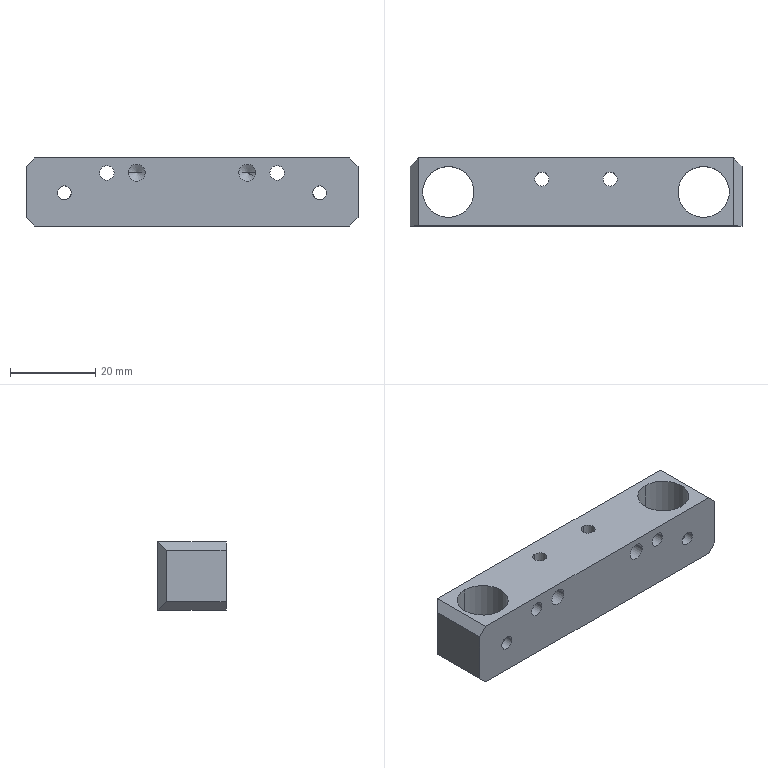Part | 1 solid | 46 faces | box 78 x 16 x 16 mm | volume 15140 mm3 | cylinder 28 | plane 14 | cone 4 | commonest cylinder face diameters 3.3 x12 3.4 x4 4 x4 6 x4 12 x4
STEP:
#1=CARTESIAN_POINT('',(15.,2.,-3.5));
#2=VERTEX_POINT('',#1);
#3=CARTESIAN_POINT('',(11.,2.,-3.5));
#4=VERTEX_POINT('',#3);
#5=CARTESIAN_POINT('',(13.,2.,-3.5));
#6=DIRECTION('',(0.,-1.,0.));
#7=DIRECTION('',(-1.,0.,0.));
#8=AXIS2_PLACEMENT_3D('',#5,#6,#7);
#9=CIRCLE('',#8,2.);
#10=EDGE_CURVE('',#2,#4,#9,.T.);
#11=ORIENTED_EDGE('',*,*,#10,.F.);
#12=CARTESIAN_POINT('',(15.,-8.,-3.5));
#13=VERTEX_POINT('',#12);
#14=CARTESIAN_POINT('',(15.,-8.,-3.5));
#15=DIRECTION('',(0.,-1.,0.));
#16=VECTOR('',#15,1000.);
#17=LINE('',#14,#16);
#18=EDGE_CURVE('',#13,#2,#17,.F.);
#19=ORIENTED_EDGE('',*,*,#18,.F.);
#20=CARTESIAN_POINT('',(11.,-8.,-3.5));
#21=VERTEX_POINT('',#20);
#22=CARTESIAN_POINT('',(13.,-8.,-3.5));
#23=DIRECTION('',(0.,-1.,0.));
#24=DIRECTION('',(-1.,0.,0.));
#25=AXIS2_PLACEMENT_3D('',#22,#23,#24);
#26=CIRCLE('',#25,2.);
#27=EDGE_CURVE('',#13,#21,#26,.T.);
#28=ORIENTED_EDGE('',*,*,#27,.T.);
#29=CARTESIAN_POINT('',(11.,-8.,-3.5));
#30=DIRECTION('',(0.,-1.,0.));
#31=VECTOR('',#30,1000.);
#32=LINE('',#29,#31);
#33=EDGE_CURVE('',#21,#4,#32,.F.);
#34=ORIENTED_EDGE('',*,*,#33,.T.);
#35=EDGE_LOOP('',(#11,#19,#28,#34));
#36=FACE_BOUND('',#35,.T.);
#37=CARTESIAN_POINT('',(13.,-8.,-3.5));
#38=DIRECTION('',(0.,-1.,0.));
#39=DIRECTION('',(1.,0.,0.));
#40=AXIS2_PLACEMENT_3D('',#37,#38,#39);
#41=CYLINDRICAL_SURFACE('',#40,2.);
#42=ADVANCED_FACE('',(#36),#41,.F.);
#43=CARTESIAN_POINT('',(13.,3.202,-3.5));
#44=VERTEX_POINT('',#43);
#45=CARTESIAN_POINT('',(11.,2.,-3.5));
#46=DIRECTION('',(-0.8572,-0.515,0.));
#47=VECTOR('',#46,1000.);
#48=LINE('',#45,#47);
#49=EDGE_CURVE('',#4,#44,#48,.F.);
#50=ORIENTED_EDGE('',*,*,#49,.T.);
#51=CARTESIAN_POINT('',(15.,2.,-3.5));
#52=DIRECTION('',(0.8572,-0.515,0.));
#53=VECTOR('',#52,1000.);
#54=LINE('',#51,#53);
#55=EDGE_CURVE('',#2,#44,#54,.F.);
#56=ORIENTED_EDGE('',*,*,#55,.F.);
#57=ORIENTED_EDGE('',*,*,#10,.T.);
#58=EDGE_LOOP('',(#50,#56,#57));
#59=FACE_BOUND('',#58,.T.);
#60=CARTESIAN_POINT('',(13.,2.,-3.5));
#61=DIRECTION('',(0.,-1.,0.));
#62=DIRECTION('',(1.,0.,0.));
#63=AXIS2_PLACEMENT_3D('',#60,#61,#62);
#64=CONICAL_SURFACE('',#63,2.,1.03);
#65=ADVANCED_FACE('',(#59),#64,.F.);
#66=CARTESIAN_POINT('',(-11.,2.,-3.5));
#67=VERTEX_POINT('',#66);
#68=CARTESIAN_POINT('',(-15.,2.,-3.5));
#69=VERTEX_POINT('',#68);
#70=CARTESIAN_POINT('',(-13.,2.,-3.5));
#71=DIRECTION('',(0.,-1.,0.));
#72=DIRECTION('',(-1.,0.,0.));
#73=AXIS2_PLACEMENT_3D('',#70,#71,#72);
#74=CIRCLE('',#73,2.);
#75=EDGE_CURVE('',#67,#69,#74,.T.);
#76=ORIENTED_EDGE('',*,*,#75,.F.);
#77=CARTESIAN_POINT('',(-11.,-8.,-3.5));
#78=VERTEX_POINT('',#77);
#79=CARTESIAN_POINT('',(-11.,-8.,-3.5));
#80=DIRECTION('',(0.,-1.,0.));
#81=VECTOR('',#80,1000.);
#82=LINE('',#79,#81);
#83=EDGE_CURVE('',#78,#67,#82,.F.);
#84=ORIENTED_EDGE('',*,*,#83,.F.);
#85=CARTESIAN_POINT('',(-15.,-8.,-3.5));
#86=VERTEX_POINT('',#85);
#87=CARTESIAN_POINT('',(-13.,-8.,-3.5));
#88=DIRECTION('',(0.,-1.,0.));
#89=DIRECTION('',(-1.,0.,0.));
#90=AXIS2_PLACEMENT_3D('',#87,#88,#89);
#91=CIRCLE('',#90,2.);
#92=EDGE_CURVE('',#78,#86,#91,.T.);
#93=ORIENTED_EDGE('',*,*,#92,.T.);
#94=CARTESIAN_POINT('',(-15.,-8.,-3.5));
#95=DIRECTION('',(0.,-1.,0.));
#96=VECTOR('',#95,1000.);
#97=LINE('',#94,#96);
#98=EDGE_CURVE('',#86,#69,#97,.F.);
#99=ORIENTED_EDGE('',*,*,#98,.T.);
#100=EDGE_LOOP('',(#76,#84,#93,#99));
#101=FACE_BOUND('',#100,.T.);
#102=CARTESIAN_POINT('',(-13.,-8.,-3.5));
#103=DIRECTION('',(0.,-1.,0.));
#104=DIRECTION('',(1.,0.,0.));
#105=AXIS2_PLACEMENT_3D('',#102,#103,#104);
#106=CYLINDRICAL_SURFACE('',#105,2.);
#107=ADVANCED_FACE('',(#101),#106,.F.);
#108=CARTESIAN_POINT('',(-13.,3.202,-3.5));
#109=VERTEX_POINT('',#108);
#110=CARTESIAN_POINT('',(-15.,2.,-3.5));
#111=DIRECTION('',(-0.8572,-0.515,0.));
#112=VECTOR('',#111,1000.);
#113=LINE('',#110,#112);
#114=EDGE_CURVE('',#69,#109,#113,.F.);
#115=ORIENTED_EDGE('',*,*,#114,.T.);
#116=CARTESIAN_POINT('',(-11.,2.,-3.5));
#117=DIRECTION('',(0.8572,-0.515,0.));
#118=VECTOR('',#117,1000.);
#119=LINE('',#116,#118);
#120=EDGE_CURVE('',#67,#109,#119,.F.);
#121=ORIENTED_EDGE('',*,*,#120,.F.);
#122=ORIENTED_EDGE('',*,*,#75,.T.);
#123=EDGE_LOOP('',(#115,#121,#122));
#124=FACE_BOUND('',#123,.T.);
#125=CARTESIAN_POINT('',(-13.,2.,-3.5));
#126=DIRECTION('',(0.,-1.,0.));
#127=DIRECTION('',(1.,0.,0.));
#128=AXIS2_PLACEMENT_3D('',#125,#126,#127);
#129=CONICAL_SURFACE('',#128,2.,1.03);
#130=ADVANCED_FACE('',(#124),#129,.F.);
#131=CARTESIAN_POINT('',(28.35,5.769,-8.2));
#132=VERTEX_POINT('',#131);
#133=CARTESIAN_POINT('',(30.,6.,-6.55));
#134=VERTEX_POINT('',#133);
#135=CARTESIAN_POINT('',(28.35,5.769,-8.2));
#136=CARTESIAN_POINT('',(28.35,5.769,-7.324));
#137=CARTESIAN_POINT('',(29.124,6.,-6.55));
#138=CARTESIAN_POINT('',(30.,6.,-6.55));
#139=B_SPLINE_CURVE_WITH_KNOTS('',3,(#135,#136,#137,#138),.UNSPECIFIED.,.F.,.F.,(4,4),(0.,0.00259),.UNSPECIFIED.);
#140=EDGE_CURVE('',#132,#134,#139,.T.);
#141=ORIENTED_EDGE('',*,*,#140,.F.);
#142=CARTESIAN_POINT('',(28.35,8.,-8.2));
#143=VERTEX_POINT('',#142);
#144=CARTESIAN_POINT('',(28.35,8.,-8.2));
#145=DIRECTION('',(0.,1.,0.));
#146=VECTOR('',#145,1000.);
#147=LINE('',#144,#146);
#148=EDGE_CURVE('',#143,#132,#147,.F.);
#149=ORIENTED_EDGE('',*,*,#148,.F.);
#150=CARTESIAN_POINT('',(31.65,8.,-8.2));
#151=VERTEX_POINT('',#150);
#152=CARTESIAN_POINT('',(30.,8.,-8.2));
#153=DIRECTION('',(0.,1.,0.));
#154=DIRECTION('',(1.,0.,0.));
#155=AXIS2_PLACEMENT_3D('',#152,#153,#154);
#156=CIRCLE('',#155,1.65);
#157=EDGE_CURVE('',#143,#151,#156,.T.);
#158=ORIENTED_EDGE('',*,*,#157,.T.);
#159=CARTESIAN_POINT('',(31.65,5.769,-8.2));
#160=VERTEX_POINT('',#159);
#161=CARTESIAN_POINT('',(31.65,8.,-8.2));
#162=DIRECTION('',(0.,1.,0.));
#163=VECTOR('',#162,1000.);
#164=LINE('',#161,#163);
#165=EDGE_CURVE('',#151,#160,#164,.F.);
#166=ORIENTED_EDGE('',*,*,#165,.T.);
#167=CARTESIAN_POINT('',(30.,6.,-6.55));
#168=CARTESIAN_POINT('',(30.876,6.,-6.55));
#169=CARTESIAN_POINT('',(31.65,5.769,-7.324));
#170=CARTESIAN_POINT('',(31.65,5.769,-8.2));
#171=B_SPLINE_CURVE_WITH_KNOTS('',3,(#167,#168,#169,#170),.UNSPECIFIED.,.F.,.F.,(4,4),(0.,0.00259),.UNSPECIFIED.);
#172=EDGE_CURVE('',#134,#160,#171,.T.);
#173=ORIENTED_EDGE('',*,*,#172,.F.);
#174=EDGE_LOOP('',(#141,#149,#158,#166,#173));
#175=FACE_BOUND('',#174,.T.);
#176=CARTESIAN_POINT('',(30.,8.,-8.2));
#177=DIRECTION('',(0.,1.,0.));
#178=DIRECTION('',(-1.,0.,0.));
#179=AXIS2_PLACEMENT_3D('',#176,#177,#178);
#180=CYLINDRICAL_SURFACE('',#179,1.65);
#181=ADVANCED_FACE('',(#175),#180,.F.);
#182=CARTESIAN_POINT('',(28.35,-8.,-8.2));
#183=VERTEX_POINT('',#182);
#184=CARTESIAN_POINT('',(31.65,-8.,-8.2));
#185=VERTEX_POINT('',#184);
#186=CARTESIAN_POINT('',(30.,-8.,-8.2));
#187=DIRECTION('',(0.,1.,0.));
#188=DIRECTION('',(1.,0.,0.));
#189=AXIS2_PLACEMENT_3D('',#186,#187,#188);
#190=CIRCLE('',#189,1.65);
#191=EDGE_CURVE('',#183,#185,#190,.T.);
#192=ORIENTED_EDGE('',*,*,#191,.F.);
#193=CARTESIAN_POINT('',(28.35,-5.769,-8.2));
#194=VERTEX_POINT('',#193);
#195=CARTESIAN_POINT('',(28.35,8.,-8.2));
#196=DIRECTION('',(0.,1.,0.));
#197=VECTOR('',#196,1000.);
#198=LINE('',#195,#197);
#199=EDGE_CURVE('',#194,#183,#198,.F.);
#200=ORIENTED_EDGE('',*,*,#199,.F.);
#201=CARTESIAN_POINT('',(30.,-6.,-6.55));
#202=VERTEX_POINT('',#201);
#203=CARTESIAN_POINT('',(30.,-6.,-6.55));
#204=CARTESIAN_POINT('',(29.124,-6.,-6.55));
#205=CARTESIAN_POINT('',(28.35,-5.769,-7.324));
#206=CARTESIAN_POINT('',(28.35,-5.769,-8.2));
#207=B_SPLINE_CURVE_WITH_KNOTS('',3,(#203,#204,#205,#206),.UNSPECIFIED.,.F.,.F.,(4,4),(0.,0.00259),.UNSPECIFIED.);
#208=EDGE_CURVE('',#202,#194,#207,.T.);
#209=ORIENTED_EDGE('',*,*,#208,.F.);
#210=CARTESIAN_POINT('',(31.65,-5.769,-8.2));
#211=VERTEX_POINT('',#210);
#212=CARTESIAN_POINT('',(31.65,-5.769,-8.2));
#213=CARTESIAN_POINT('',(31.65,-5.769,-7.324));
#214=CARTESIAN_POINT('',(30.876,-6.,-6.55));
#215=CARTESIAN_POINT('',(30.,-6.,-6.55));
#216=B_SPLINE_CURVE_WITH_KNOTS('',3,(#212,#213,#214,#215),.UNSPECIFIED.,.F.,.F.,(4,4),(0.,0.00259),.UNSPECIFIED.);
#217=EDGE_CURVE('',#211,#202,#216,.T.);
#218=ORIENTED_EDGE('',*,*,#217,.F.);
#219=CARTESIAN_POINT('',(31.65,8.,-8.2));
#220=DIRECTION('',(0.,1.,0.));
#221=VECTOR('',#220,1000.);
#222=LINE('',#219,#221);
#223=EDGE_CURVE('',#211,#185,#222,.F.);
#224=ORIENTED_EDGE('',*,*,#223,.T.);
#225=EDGE_LOOP('',(#192,#200,#209,#218,#224));
#226=FACE_BOUND('',#225,.T.);
#227=CARTESIAN_POINT('',(30.,8.,-8.2));
#228=DIRECTION('',(0.,1.,0.));
#229=DIRECTION('',(-1.,0.,0.));
#230=AXIS2_PLACEMENT_3D('',#227,#228,#229);
#231=CYLINDRICAL_SURFACE('',#230,1.65);
#232=ADVANCED_FACE('',(#226),#231,.F.);
#233=CARTESIAN_POINT('',(-31.65,5.769,-8.2));
#234=VERTEX_POINT('',#233);
#235=CARTESIAN_POINT('',(-30.,6.,-6.55));
#236=VERTEX_POINT('',#235);
#237=CARTESIAN_POINT('',(-31.65,5.769,-8.2));
#238=CARTESIAN_POINT('',(-31.65,5.769,-7.324));
#239=CARTESIAN_POINT('',(-30.876,6.,-6.55));
#240=CARTESIAN_POINT('',(-30.,6.,-6.55));
#241=B_SPLINE_CURVE_WITH_KNOTS('',3,(#237,#238,#239,#240),.UNSPECIFIED.,.F.,.F.,(4,4),(0.,0.00259),.UNSPECIFIED.);
#242=EDGE_CURVE('',#234,#236,#241,.T.);
#243=ORIENTED_EDGE('',*,*,#242,.F.);
#244=CARTESIAN_POINT('',(-31.65,8.,-8.2));
#245=VERTEX_POINT('',#244);
#246=CARTESIAN_POINT('',(-31.65,8.,-8.2));
#247=DIRECTION('',(0.,1.,0.));
#248=VECTOR('',#247,1000.);
#249=LINE('',#246,#248);
#250=EDGE_CURVE('',#245,#234,#249,.F.);
#251=ORIENTED_EDGE('',*,*,#250,.F.);
#252=CARTESIAN_POINT('',(-28.35,8.,-8.2));
#253=VERTEX_POINT('',#252);
#254=CARTESIAN_POINT('',(-30.,8.,-8.2));
#255=DIRECTION('',(0.,1.,0.));
#256=DIRECTION('',(1.,0.,0.));
#257=AXIS2_PLACEMENT_3D('',#254,#255,#256);
#258=CIRCLE('',#257,1.65);
#259=EDGE_CURVE('',#245,#253,#258,.T.);
#260=ORIENTED_EDGE('',*,*,#259,.T.);
#261=CARTESIAN_POINT('',(-28.35,5.769,-8.2));
#262=VERTEX_POINT('',#261);
#263=CARTESIAN_POINT('',(-28.35,8.,-8.2));
#264=DIRECTION('',(0.,1.,0.));
#265=VECTOR('',#264,1000.);
#266=LINE('',#263,#265);
#267=EDGE_CURVE('',#253,#262,#266,.F.);
#268=ORIENTED_EDGE('',*,*,#267,.T.);
#269=CARTESIAN_POINT('',(-30.,6.,-6.55));
#270=CARTESIAN_POINT('',(-29.124,6.,-6.55));
#271=CARTESIAN_POINT('',(-28.35,5.769,-7.324));
#272=CARTESIAN_POINT('',(-28.35,5.769,-8.2));
#273=B_SPLINE_CURVE_WITH_KNOTS('',3,(#269,#270,#271,#272),.UNSPECIFIED.,.F.,.F.,(4,4),(0.,0.00259),.UNSPECIFIED.);
#274=EDGE_CURVE('',#236,#262,#273,.T.);
#275=ORIENTED_EDGE('',*,*,#274,.F.);
#276=EDGE_LOOP('',(#243,#251,#260,#268,#275));
#277=FACE_BOUND('',#276,.T.);
#278=CARTESIAN_POINT('',(-30.,8.,-8.2));
#279=DIRECTION('',(0.,1.,0.));
#280=DIRECTION('',(-1.,0.,0.));
#281=AXIS2_PLACEMENT_3D('',#278,#279,#280);
#282=CYLINDRICAL_SURFACE('',#281,1.65);
#283=ADVANCED_FACE('',(#277),#282,.F.);
#284=CARTESIAN_POINT('',(-31.65,-8.,-8.2));
#285=VERTEX_POINT('',#284);
#286=CARTESIAN_POINT('',(-28.35,-8.,-8.2));
#287=VERTEX_POINT('',#286);
#288=CARTESIAN_POINT('',(-30.,-8.,-8.2));
#289=DIRECTION('',(0.,1.,0.));
#290=DIRECTION('',(1.,0.,0.));
#291=AXIS2_PLACEMENT_3D('',#288,#289,#290);
#292=CIRCLE('',#291,1.65);
#293=EDGE_CURVE('',#285,#287,#292,.T.);
#294=ORIENTED_EDGE('',*,*,#293,.F.);
#295=CARTESIAN_POINT('',(-31.65,-5.769,-8.2));
#296=VERTEX_POINT('',#295);
#297=CARTESIAN_POINT('',(-31.65,8.,-8.2));
#298=DIRECTION('',(0.,1.,0.));
#299=VECTOR('',#298,1000.);
#300=LINE('',#297,#299);
#301=EDGE_CURVE('',#296,#285,#300,.F.);
#302=ORIENTED_EDGE('',*,*,#301,.F.);
#303=CARTESIAN_POINT('',(-30.,-6.,-6.55));
#304=VERTEX_POINT('',#303);
#305=CARTESIAN_POINT('',(-30.,-6.,-6.55));
#306=CARTESIAN_POINT('',(-30.876,-6.,-6.55));
#307=CARTESIAN_POINT('',(-31.65,-5.769,-7.324));
#308=CARTESIAN_POINT('',(-31.65,-5.769,-8.2));
#309=B_SPLINE_CURVE_WITH_KNOTS('',3,(#305,#306,#307,#308),.UNSPECIFIED.,.F.,.F.,(4,4),(0.,0.00259),.UNSPECIFIED.);
#310=EDGE_CURVE('',#304,#296,#309,.T.);
#311=ORIENTED_EDGE('',*,*,#310,.F.);
#312=CARTESIAN_POINT('',(-28.35,-5.769,-8.2));
#313=VERTEX_POINT('',#312);
#314=CARTESIAN_POINT('',(-28.35,-5.769,-8.2));
#315=CARTESIAN_POINT('',(-28.35,-5.769,-7.324));
#316=CARTESIAN_POINT('',(-29.124,-6.,-6.55));
#317=CARTESIAN_POINT('',(-30.,-6.,-6.55));
#318=B_SPLINE_CURVE_WITH_KNOTS('',3,(#314,#315,#316,#317),.UNSPECIFIED.,.F.,.F.,(4,4),(0.,0.00259),.UNSPECIFIED.);
#319=EDGE_CURVE('',#313,#304,#318,.T.);
#320=ORIENTED_EDGE('',*,*,#319,.F.);
#321=CARTESIAN_POINT('',(-28.35,8.,-8.2));
#322=DIRECTION('',(0.,1.,0.));
#323=VECTOR('',#322,1000.);
#324=LINE('',#321,#323);
#325=EDGE_CURVE('',#313,#287,#324,.F.);
#326=ORIENTED_EDGE('',*,*,#325,.T.);
#327=EDGE_LOOP('',(#294,#302,#311,#320,#326));
#328=FACE_BOUND('',#327,.T.);
#329=CARTESIAN_POINT('',(-30.,8.,-8.2));
#330=DIRECTION('',(0.,1.,0.));
#331=DIRECTION('',(-1.,0.,0.));
#332=AXIS2_PLACEMENT_3D('',#329,#330,#331);
#333=CYLINDRICAL_SURFACE('',#332,1.65);
#334=ADVANCED_FACE('',(#328),#333,.F.);
#335=CARTESIAN_POINT('',(17.,4.6,-3.5));
#336=VERTEX_POINT('',#335);
#337=CARTESIAN_POINT('',(23.,4.6,-3.5));
#338=VERTEX_POINT('',#337);
#339=CARTESIAN_POINT('',(20.,4.6,-3.5));
#340=DIRECTION('',(0.,1.,0.));
#341=DIRECTION('',(1.,0.,0.));
#342=AXIS2_PLACEMENT_3D('',#339,#340,#341);
#343=CIRCLE('',#342,3.);
#344=EDGE_CURVE('',#336,#338,#343,.T.);
#345=ORIENTED_EDGE('',*,*,#344,.F.);
#346=CARTESIAN_POINT('',(17.,8.,-3.5));
#347=VERTEX_POINT('',#346);
#348=CARTESIAN_POINT('',(17.,8.,-3.5));
#349=DIRECTION('',(0.,1.,0.));
#350=VECTOR('',#349,1000.);
#351=LINE('',#348,#350);
#352=EDGE_CURVE('',#347,#336,#351,.F.);
#353=ORIENTED_EDGE('',*,*,#352,.F.);
#354=CARTESIAN_POINT('',(23.,8.,-3.5));
#355=VERTEX_POINT('',#354);
#356=CARTESIAN_POINT('',(20.,8.,-3.5));
#357=DIRECTION('',(0.,1.,0.));
#358=DIRECTION('',(1.,0.,0.));
#359=AXIS2_PLACEMENT_3D('',#356,#357,#358);
#360=CIRCLE('',#359,3.);
#361=EDGE_CURVE('',#347,#355,#360,.T.);
#362=ORIENTED_EDGE('',*,*,#361,.T.);
#363=CARTESIAN_POINT('',(23.,8.,-3.5));
#364=DIRECTION('',(0.,1.,0.));
#365=VECTOR('',#364,1000.);
#366=LINE('',#363,#365);
#367=EDGE_CURVE('',#355,#338,#366,.F.);
#368=ORIENTED_EDGE('',*,*,#367,.T.);
#369=EDGE_LOOP('',(#345,#353,#362,#368));
#370=FACE_BOUND('',#369,.T.);
#371=CARTESIAN_POINT('',(20.,8.,-3.5));
#372=DIRECTION('',(0.,1.,0.));
#373=DIRECTION('',(-1.,0.,0.));
#374=AXIS2_PLACEMENT_3D('',#371,#372,#373);
#375=CYLINDRICAL_SURFACE('',#374,3.);
#376=ADVANCED_FACE('',(#370),#375,.F.);
#377=CARTESIAN_POINT('',(18.3,-8.,-3.5));
#378=VERTEX_POINT('',#377);
#379=CARTESIAN_POINT('',(21.7,-8.,-3.5));
#380=VERTEX_POINT('',#379);
#381=CARTESIAN_POINT('',(20.,-8.,-3.5));
#382=DIRECTION('',(0.,1.,0.));
#383=DIRECTION('',(1.,0.,0.));
#384=AXIS2_PLACEMENT_3D('',#381,#382,#383);
#385=CIRCLE('',#384,1.7);
#386=EDGE_CURVE('',#378,#380,#385,.T.);
#387=ORIENTED_EDGE('',*,*,#386,.F.);
#388=CARTESIAN_POINT('',(18.3,4.6,-3.5));
#389=VERTEX_POINT('',#388);
#390=CARTESIAN_POINT('',(18.3,8.,-3.5));
#391=DIRECTION('',(0.,1.,0.));
#392=VECTOR('',#391,1000.);
#393=LINE('',#390,#392);
#394=EDGE_CURVE('',#389,#378,#393,.F.);
#395=ORIENTED_EDGE('',*,*,#394,.F.);
#396=CARTESIAN_POINT('',(21.7,4.6,-3.5));
#397=VERTEX_POINT('',#396);
#398=CARTESIAN_POINT('',(20.,4.6,-3.5));
#399=DIRECTION('',(0.,1.,0.));
#400=DIRECTION('',(1.,0.,0.));
#401=AXIS2_PLACEMENT_3D('',#398,#399,#400);
#402=CIRCLE('',#401,1.7);
#403=EDGE_CURVE('',#389,#397,#402,.T.);
#404=ORIENTED_EDGE('',*,*,#403,.T.);
#405=CARTESIAN_POINT('',(21.7,8.,-3.5));
#406=DIRECTION('',(0.,1.,0.));
#407=VECTOR('',#406,1000.);
#408=LINE('',#405,#407);
#409=EDGE_CURVE('',#397,#380,#408,.F.);
#410=ORIENTED_EDGE('',*,*,#409,.T.);
#411=EDGE_LOOP('',(#387,#395,#404,#410));
#412=FACE_BOUND('',#411,.T.);
#413=CARTESIAN_POINT('',(20.,8.,-3.5));
#414=DIRECTION('',(0.,1.,0.));
#415=DIRECTION('',(-1.,0.,0.));
#416=AXIS2_PLACEMENT_3D('',#413,#414,#415);
#417=CYLINDRICAL_SURFACE('',#416,1.7);
#418=ADVANCED_FACE('',(#412),#417,.F.);
#419=CARTESIAN_POINT('',(-23.,4.6,-3.5));
#420=VERTEX_POINT('',#419);
#421=CARTESIAN_POINT('',(-17.,4.6,-3.5));
#422=VERTEX_POINT('',#421);
#423=CARTESIAN_POINT('',(-20.,4.6,-3.5));
#424=DIRECTION('',(0.,1.,0.));
#425=DIRECTION('',(1.,0.,0.));
#426=AXIS2_PLACEMENT_3D('',#423,#424,#425);
#427=CIRCLE('',#426,3.);
#428=EDGE_CURVE('',#420,#422,#427,.T.);
#429=ORIENTED_EDGE('',*,*,#428,.F.);
#430=CARTESIAN_POINT('',(-23.,8.,-3.5));
#431=VERTEX_POINT('',#430);
#432=CARTESIAN_POINT('',(-23.,8.,-3.5));
#433=DIRECTION('',(0.,1.,0.));
#434=VECTOR('',#433,1000.);
#435=LINE('',#432,#434);
#436=EDGE_CURVE('',#431,#420,#435,.F.);
#437=ORIENTED_EDGE('',*,*,#436,.F.);
#438=CARTESIAN_POINT('',(-17.,8.,-3.5));
#439=VERTEX_POINT('',#438);
#440=CARTESIAN_POINT('',(-20.,8.,-3.5));
#441=DIRECTION('',(0.,1.,0.));
#442=DIRECTION('',(1.,0.,0.));
#443=AXIS2_PLACEMENT_3D('',#440,#441,#442);
#444=CIRCLE('',#443,3.);
#445=EDGE_CURVE('',#431,#439,#444,.T.);
#446=ORIENTED_EDGE('',*,*,#445,.T.);
#447=CARTESIAN_POINT('',(-17.,8.,-3.5));
#448=DIRECTION('',(0.,1.,0.));
#449=VECTOR('',#448,1000.);
#450=LINE('',#447,#449);
#451=EDGE_CURVE('',#439,#422,#450,.F.);
#452=ORIENTED_EDGE('',*,*,#451,.T.);
#453=EDGE_LOOP('',(#429,#437,#446,#452));
#454=FACE_BOUND('',#453,.T.);
#455=CARTESIAN_POINT('',(-20.,8.,-3.5));
#456=DIRECTION('',(0.,1.,0.));
#457=DIRECTION('',(-1.,0.,0.));
#458=AXIS2_PLACEMENT_3D('',#455,#456,#457);
#459=CYLINDRICAL_SURFACE('',#458,3.);
#460=ADVANCED_FACE('',(#454),#459,.F.);
#461=CARTESIAN_POINT('',(-21.7,-8.,-3.5));
#462=VERTEX_POINT('',#461);
#463=CARTESIAN_POINT('',(-18.3,-8.,-3.5));
#464=VERTEX_POINT('',#463);
#465=CARTESIAN_POINT('',(-20.,-8.,-3.5));
#466=DIRECTION('',(0.,1.,0.));
#467=DIRECTION('',(1.,0.,0.));
#468=AXIS2_PLACEMENT_3D('',#465,#466,#467);
#469=CIRCLE('',#468,1.7);
#470=EDGE_CURVE('',#462,#464,#469,.T.);
#471=ORIENTED_EDGE('',*,*,#470,.F.);
#472=CARTESIAN_POINT('',(-21.7,4.6,-3.5));
#473=VERTEX_POINT('',#472);
#474=CARTESIAN_POINT('',(-21.7,8.,-3.5));
#475=DIRECTION('',(0.,1.,0.));
#476=VECTOR('',#475,1000.);
#477=LINE('',#474,#476);
#478=EDGE_CURVE('',#473,#462,#477,.F.);
#479=ORIENTED_EDGE('',*,*,#478,.F.);
#480=CARTESIAN_POINT('',(-18.3,4.6,-3.5));
#481=VERTEX_POINT('',#480);
#482=CARTESIAN_POINT('',(-20.,4.6,-3.5));
#483=DIRECTION('',(0.,1.,0.));
#484=DIRECTION('',(1.,0.,0.));
#485=AXIS2_PLACEMENT_3D('',#482,#483,#484);
#486=CIRCLE('',#485,1.7);
#487=EDGE_CURVE('',#473,#481,#486,.T.);
#488=ORIENTED_EDGE('',*,*,#487,.T.);
#489=CARTESIAN_POINT('',(-18.3,8.,-3.5));
#490=DIRECTION('',(0.,1.,0.));
#491=VECTOR('',#490,1000.);
#492=LINE('',#489,#491);
#493=EDGE_CURVE('',#481,#464,#492,.F.);
#494=ORIENTED_EDGE('',*,*,#493,.T.);
#495=EDGE_LOOP('',(#471,#479,#488,#494));
#496=FACE_BOUND('',#495,.T.);
#497=CARTESIAN_POINT('',(-20.,8.,-3.5));
#498=DIRECTION('',(0.,1.,0.));
#499=DIRECTION('',(-1.,0.,0.));
#500=AXIS2_PLACEMENT_3D('',#497,#498,#499);
#501=CYLINDRICAL_SURFACE('',#500,1.7);
#502=ADVANCED_FACE('',(#496),#501,.F.);
#503=CARTESIAN_POINT('',(8.,1.35,-16.));
#504=VERTEX_POINT('',#503);
#505=CARTESIAN_POINT('',(8.,4.65,-16.));
#506=VERTEX_POINT('',#505);
#507=CARTESIAN_POINT('',(8.,3.,-16.));
#508=DIRECTION('',(0.,0.,1.));
#509=DIRECTION('',(0.,1.,0.));
#510=AXIS2_PLACEMENT_3D('',#507,#508,#509);
#511=CIRCLE('',#510,1.65);
#512=EDGE_CURVE('',#504,#506,#511,.T.);
#513=ORIENTED_EDGE('',*,*,#512,.F.);
#514=CARTESIAN_POINT('',(8.,1.35,0.));
#515=VERTEX_POINT('',#514);
#516=CARTESIAN_POINT('',(8.,1.35,0.));
#517=DIRECTION('',(0.,0.,1.));
#518=VECTOR('',#517,1000.);
#519=LINE('',#516,#518);
#520=EDGE_CURVE('',#515,#504,#519,.F.);
#521=ORIENTED_EDGE('',*,*,#520,.F.);
#522=CARTESIAN_POINT('',(8.,4.65,0.));
#523=VERTEX_POINT('',#522);
#524=CARTESIAN_POINT('',(8.,3.,0.));
#525=DIRECTION('',(0.,0.,1.));
#526=DIRECTION('',(0.,1.,0.));
#527=AXIS2_PLACEMENT_3D('',#524,#525,#526);
#528=CIRCLE('',#527,1.65);
#529=EDGE_CURVE('',#515,#523,#528,.T.);
#530=ORIENTED_EDGE('',*,*,#529,.T.);
#531=CARTESIAN_POINT('',(8.,4.65,0.));
#532=DIRECTION('',(0.,0.,1.));
#533=VECTOR('',#532,1000.);
#534=LINE('',#531,#533);
#535=EDGE_CURVE('',#523,#506,#534,.F.);
#536=ORIENTED_EDGE('',*,*,#535,.T.);
#537=EDGE_LOOP('',(#513,#521,#530,#536));
#538=FACE_BOUND('',#537,.T.);
#539=CARTESIAN_POINT('',(8.,3.,0.));
#540=DIRECTION('',(0.,0.,1.));
#541=DIRECTION('',(0.,-1.,0.));
#542=AXIS2_PLACEMENT_3D('',#539,#540,#541);
#543=CYLINDRICAL_SURFACE('',#542,1.65);
#544=ADVANCED_FACE('',(#538),#543,.F.);
#545=CARTESIAN_POINT('',(-8.,1.35,-16.));
#546=VERTEX_POINT('',#545);
#547=CARTESIAN_POINT('',(-8.,4.65,-16.));
#548=VERTEX_POINT('',#547);
#549=CARTESIAN_POINT('',(-8.,3.,-16.));
#550=DIRECTION('',(0.,0.,1.));
#551=DIRECTION('',(0.,1.,0.));
#552=AXIS2_PLACEMENT_3D('',#549,#550,#551);
#553=CIRCLE('',#552,1.65);
#554=EDGE_CURVE('',#546,#548,#553,.T.);
#555=ORIENTED_EDGE('',*,*,#554,.F.);
#556=CARTESIAN_POINT('',(-8.,1.35,0.));
#557=VERTEX_POINT('',#556);
#558=CARTESIAN_POINT('',(-8.,1.35,0.));
#559=DIRECTION('',(0.,0.,1.));
#560=VECTOR('',#559,1000.);
#561=LINE('',#558,#560);
#562=EDGE_CURVE('',#557,#546,#561,.F.);
#563=ORIENTED_EDGE('',*,*,#562,.F.);
#564=CARTESIAN_POINT('',(-8.,4.65,0.));
#565=VERTEX_POINT('',#564);
#566=CARTESIAN_POINT('',(-8.,3.,0.));
#567=DIRECTION('',(0.,0.,1.));
#568=DIRECTION('',(0.,1.,0.));
#569=AXIS2_PLACEMENT_3D('',#566,#567,#568);
#570=CIRCLE('',#569,1.65);
#571=EDGE_CURVE('',#557,#565,#570,.T.);
#572=ORIENTED_EDGE('',*,*,#571,.T.);
#573=CARTESIAN_POINT('',(-8.,4.65,0.));
#574=DIRECTION('',(0.,0.,1.));
#575=VECTOR('',#574,1000.);
#576=LINE('',#573,#575);
#577=EDGE_CURVE('',#565,#548,#576,.F.);
#578=ORIENTED_EDGE('',*,*,#577,.T.);
#579=EDGE_LOOP('',(#555,#563,#572,#578));
#580=FACE_BOUND('',#579,.T.);
#581=CARTESIAN_POINT('',(-8.,3.,0.));
#582=DIRECTION('',(0.,0.,1.));
#583=DIRECTION('',(0.,-1.,0.));
#584=AXIS2_PLACEMENT_3D('',#581,#582,#583);
#585=CYLINDRICAL_SURFACE('',#584,1.65);
#586=ADVANCED_FACE('',(#580),#585,.F.);
#587=CARTESIAN_POINT('',(-30.,-6.,-16.));
#588=VERTEX_POINT('',#587);
#589=CARTESIAN_POINT('',(-30.,6.,-16.));
#590=VERTEX_POINT('',#589);
#591=CARTESIAN_POINT('',(-30.,0.,-16.));
#592=DIRECTION('',(0.,0.,1.));
#593=DIRECTION('',(0.,1.,0.));
#594=AXIS2_PLACEMENT_3D('',#591,#592,#593);
#595=CIRCLE('',#594,6.);
#596=EDGE_CURVE('',#588,#590,#595,.T.);
#597=ORIENTED_EDGE('',*,*,#596,.F.);
#598=CARTESIAN_POINT('',(-30.,-6.,-9.85));
#599=VERTEX_POINT('',#598);
#600=CARTESIAN_POINT('',(-30.,-6.,0.));
#601=DIRECTION('',(0.,0.,1.));
#602=VECTOR('',#601,1000.);
#603=LINE('',#600,#602);
#604=EDGE_CURVE('',#599,#588,#603,.F.);
#605=ORIENTED_EDGE('',*,*,#604,.F.);
#606=CARTESIAN_POINT('',(-30.,-6.,-9.85));
#607=CARTESIAN_POINT('',(-29.124,-6.,-9.85));
#608=CARTESIAN_POINT('',(-28.35,-5.769,-9.076));
#609=CARTESIAN_POINT('',(-28.35,-5.769,-8.2));
#610=B_SPLINE_CURVE_WITH_KNOTS('',3,(#606,#607,#608,#609),.UNSPECIFIED.,.F.,.F.,(4,4),(0.,0.00259),.UNSPECIFIED.);
#611=EDGE_CURVE('',#599,#313,#610,.T.);
#612=ORIENTED_EDGE('',*,*,#611,.T.);
#613=ORIENTED_EDGE('',*,*,#319,.T.);
#614=CARTESIAN_POINT('',(-30.,-6.,0.));
#615=VERTEX_POINT('',#614);
#616=CARTESIAN_POINT('',(-30.,-6.,0.));
#617=DIRECTION('',(0.,0.,1.));
#618=VECTOR('',#617,1000.);
#619=LINE('',#616,#618);
#620=EDGE_CURVE('',#304,#615,#619,.T.);
#621=ORIENTED_EDGE('',*,*,#620,.T.);
#622=CARTESIAN_POINT('',(-30.,6.,0.));
#623=VERTEX_POINT('',#622);
#624=CARTESIAN_POINT('',(-30.,0.,0.));
#625=DIRECTION('',(0.,0.,1.));
#626=DIRECTION('',(0.,1.,0.));
#627=AXIS2_PLACEMENT_3D('',#624,#625,#626);
#628=CIRCLE('',#627,6.);
#629=EDGE_CURVE('',#615,#623,#628,.T.);
#630=ORIENTED_EDGE('',*,*,#629,.T.);
#631=CARTESIAN_POINT('',(-30.,6.,0.));
#632=DIRECTION('',(0.,0.,1.));
#633=VECTOR('',#632,1000.);
#634=LINE('',#631,#633);
#635=EDGE_CURVE('',#623,#236,#634,.F.);
#636=ORIENTED_EDGE('',*,*,#635,.T.);
#637=ORIENTED_EDGE('',*,*,#274,.T.);
#638=CARTESIAN_POINT('',(-30.,6.,-9.85));
#639=VERTEX_POINT('',#638);
#640=CARTESIAN_POINT('',(-28.35,5.769,-8.2));
#641=CARTESIAN_POINT('',(-28.35,5.769,-9.076));
#642=CARTESIAN_POINT('',(-29.124,6.,-9.85));
#643=CARTESIAN_POINT('',(-30.,6.,-9.85));
#644=B_SPLINE_CURVE_WITH_KNOTS('',3,(#640,#641,#642,#643),.UNSPECIFIED.,.F.,.F.,(4,4),(0.,0.00259),.UNSPECIFIED.);
#645=EDGE_CURVE('',#262,#639,#644,.T.);
#646=ORIENTED_EDGE('',*,*,#645,.T.);
#647=CARTESIAN_POINT('',(-30.,6.,0.));
#648=DIRECTION('',(0.,0.,1.));
#649=VECTOR('',#648,1000.);
#650=LINE('',#647,#649);
#651=EDGE_CURVE('',#590,#639,#650,.T.);
#652=ORIENTED_EDGE('',*,*,#651,.F.);
#653=EDGE_LOOP('',(#597,#605,#612,#613,#621,#630,#636,#637,#646,#652));
#654=FACE_BOUND('',#653,.T.);
#655=CARTESIAN_POINT('',(-30.,0.,0.));
#656=DIRECTION('',(0.,0.,1.));
#657=DIRECTION('',(0.,-1.,0.));
#658=AXIS2_PLACEMENT_3D('',#655,#656,#657);
#659=CYLINDRICAL_SURFACE('',#658,6.);
#660=ADVANCED_FACE('',(#654),#659,.F.);
#661=CARTESIAN_POINT('',(30.,-6.,-16.));
#662=VERTEX_POINT('',#661);
#663=CARTESIAN_POINT('',(30.,6.,-16.));
#664=VERTEX_POINT('',#663);
#665=CARTESIAN_POINT('',(30.,0.,-16.));
#666=DIRECTION('',(0.,0.,1.));
#667=DIRECTION('',(0.,1.,0.));
#668=AXIS2_PLACEMENT_3D('',#665,#666,#667);
#669=CIRCLE('',#668,6.);
#670=EDGE_CURVE('',#662,#664,#669,.T.);
#671=ORIENTED_EDGE('',*,*,#670,.F.);
#672=CARTESIAN_POINT('',(30.,-6.,-9.85));
#673=VERTEX_POINT('',#672);
#674=CARTESIAN_POINT('',(30.,-6.,0.));
#675=DIRECTION('',(0.,0.,1.));
#676=VECTOR('',#675,1000.);
#677=LINE('',#674,#676);
#678=EDGE_CURVE('',#673,#662,#677,.F.);
#679=ORIENTED_EDGE('',*,*,#678,.F.);
#680=CARTESIAN_POINT('',(30.,-6.,-9.85));
#681=CARTESIAN_POINT('',(30.876,-6.,-9.85));
#682=CARTESIAN_POINT('',(31.65,-5.769,-9.076));
#683=CARTESIAN_POINT('',(31.65,-5.769,-8.2));
#684=B_SPLINE_CURVE_WITH_KNOTS('',3,(#680,#681,#682,#683),.UNSPECIFIED.,.F.,.F.,(4,4),(0.,0.00259),.UNSPECIFIED.);
#685=EDGE_CURVE('',#673,#211,#684,.T.);
#686=ORIENTED_EDGE('',*,*,#685,.T.);
#687=ORIENTED_EDGE('',*,*,#217,.T.);
#688=CARTESIAN_POINT('',(30.,-6.,0.));
#689=VERTEX_POINT('',#688);
#690=CARTESIAN_POINT('',(30.,-6.,0.));
#691=DIRECTION('',(0.,0.,1.));
#692=VECTOR('',#691,1000.);
#693=LINE('',#690,#692);
#694=EDGE_CURVE('',#202,#689,#693,.T.);
#695=ORIENTED_EDGE('',*,*,#694,.T.);
#696=CARTESIAN_POINT('',(30.,6.,0.));
#697=VERTEX_POINT('',#696);
#698=CARTESIAN_POINT('',(30.,0.,0.));
#699=DIRECTION('',(0.,0.,1.));
#700=DIRECTION('',(0.,1.,0.));
#701=AXIS2_PLACEMENT_3D('',#698,#699,#700);
#702=CIRCLE('',#701,6.);
#703=EDGE_CURVE('',#689,#697,#702,.T.);
#704=ORIENTED_EDGE('',*,*,#703,.T.);
#705=CARTESIAN_POINT('',(30.,6.,0.));
#706=DIRECTION('',(0.,0.,1.));
#707=VECTOR('',#706,1000.);
#708=LINE('',#705,#707);
#709=EDGE_CURVE('',#697,#134,#708,.F.);
#710=ORIENTED_EDGE('',*,*,#709,.T.);
#711=ORIENTED_EDGE('',*,*,#172,.T.);
#712=CARTESIAN_POINT('',(30.,6.,-9.85));
#713=VERTEX_POINT('',#712);
#714=CARTESIAN_POINT('',(31.65,5.769,-8.2));
#715=CARTESIAN_POINT('',(31.65,5.769,-9.076));
#716=CARTESIAN_POINT('',(30.876,6.,-9.85));
#717=CARTESIAN_POINT('',(30.,6.,-9.85));
#718=B_SPLINE_CURVE_WITH_KNOTS('',3,(#714,#715,#716,#717),.UNSPECIFIED.,.F.,.F.,(4,4),(0.,0.00259),.UNSPECIFIED.);
#719=EDGE_CURVE('',#160,#713,#718,.T.);
#720=ORIENTED_EDGE('',*,*,#719,.T.);
#721=CARTESIAN_POINT('',(30.,6.,0.));
#722=DIRECTION('',(0.,0.,1.));
#723=VECTOR('',#722,1000.);
#724=LINE('',#721,#723);
#725=EDGE_CURVE('',#664,#713,#724,.T.);
#726=ORIENTED_EDGE('',*,*,#725,.F.);
#727=EDGE_LOOP('',(#671,#679,#686,#687,#695,#704,#710,#711,#720,#726));
#728=FACE_BOUND('',#727,.T.);
#729=CARTESIAN_POINT('',(30.,0.,0.));
#730=DIRECTION('',(0.,0.,1.));
#731=DIRECTION('',(0.,-1.,0.));
#732=AXIS2_PLACEMENT_3D('',#729,#730,#731);
#733=CYLINDRICAL_SURFACE('',#732,6.);
#734=ADVANCED_FACE('',(#728),#733,.F.);
#735=CARTESIAN_POINT('',(-39.,6.,-2.));
#736=VERTEX_POINT('',#735);
#737=CARTESIAN_POINT('',(-39.,6.,-14.));
#738=VERTEX_POINT('',#737);
#739=CARTESIAN_POINT('',(-39.,6.,-16.));
#740=DIRECTION('',(0.,0.,-1.));
#741=VECTOR('',#740,1000.);
#742=LINE('',#739,#741);
#743=EDGE_CURVE('',#736,#738,#742,.T.);
#744=ORIENTED_EDGE('',*,*,#743,.T.);
#745=CARTESIAN_POINT('',(-39.,-8.,-14.));
#746=VERTEX_POINT('',#745);
#747=CARTESIAN_POINT('',(-39.,-8.,-14.));
#748=DIRECTION('',(0.,-1.,0.));
#749=VECTOR('',#748,1000.);
#750=LINE('',#747,#749);
#751=EDGE_CURVE('',#738,#746,#750,.T.);
#752=ORIENTED_EDGE('',*,*,#751,.T.);
#753=CARTESIAN_POINT('',(-39.,-8.,-2.));
#754=VERTEX_POINT('',#753);
#755=CARTESIAN_POINT('',(-39.,-8.,-16.));
#756=DIRECTION('',(0.,0.,1.));
#757=VECTOR('',#756,1000.);
#758=LINE('',#755,#757);
#759=EDGE_CURVE('',#746,#754,#758,.T.);
#760=ORIENTED_EDGE('',*,*,#759,.T.);
#761=CARTESIAN_POINT('',(-39.,8.,-2.));
#762=DIRECTION('',(0.,1.,0.));
#763=VECTOR('',#762,1000.);
#764=LINE('',#761,#763);
#765=EDGE_CURVE('',#754,#736,#764,.T.);
#766=ORIENTED_EDGE('',*,*,#765,.T.);
#767=EDGE_LOOP('',(#744,#752,#760,#766));
#768=FACE_BOUND('',#767,.T.);
#769=CARTESIAN_POINT('',(-39.,8.,-16.));
#770=DIRECTION('',(1.,0.,0.));
#771=DIRECTION('',(0.,1.,0.));
#772=AXIS2_PLACEMENT_3D('',#769,#770,#771);
#773=PLANE('',#772);
#774=ADVANCED_FACE('',(#768),#773,.F.);
#775=CARTESIAN_POINT('',(30.,8.,-8.2));
#776=DIRECTION('',(0.,1.,0.));
#777=DIRECTION('',(1.,0.,0.));
#778=AXIS2_PLACEMENT_3D('',#775,#776,#777);
#779=CIRCLE('',#778,1.65);
#780=EDGE_CURVE('',#151,#143,#779,.T.);
#781=ORIENTED_EDGE('',*,*,#780,.F.);
#782=ORIENTED_EDGE('',*,*,#157,.F.);
#783=EDGE_LOOP('',(#781,#782));
#784=FACE_BOUND('',#783,.T.);
#785=CARTESIAN_POINT('',(-30.,8.,-8.2));
#786=DIRECTION('',(0.,1.,0.));
#787=DIRECTION('',(1.,0.,0.));
#788=AXIS2_PLACEMENT_3D('',#785,#786,#787);
#789=CIRCLE('',#788,1.65);
#790=EDGE_CURVE('',#253,#245,#789,.T.);
#791=ORIENTED_EDGE('',*,*,#790,.F.);
#792=ORIENTED_EDGE('',*,*,#259,.F.);
#793=EDGE_LOOP('',(#791,#792));
#794=FACE_BOUND('',#793,.T.);
#795=CARTESIAN_POINT('',(20.,8.,-3.5));
#796=DIRECTION('',(0.,1.,0.));
#797=DIRECTION('',(1.,0.,0.));
#798=AXIS2_PLACEMENT_3D('',#795,#796,#797);
#799=CIRCLE('',#798,3.);
#800=EDGE_CURVE('',#355,#347,#799,.T.);
#801=ORIENTED_EDGE('',*,*,#800,.F.);
#802=ORIENTED_EDGE('',*,*,#361,.F.);
#803=EDGE_LOOP('',(#801,#802));
#804=FACE_BOUND('',#803,.T.);
#805=CARTESIAN_POINT('',(-20.,8.,-3.5));
#806=DIRECTION('',(0.,1.,0.));
#807=DIRECTION('',(1.,0.,0.));
#808=AXIS2_PLACEMENT_3D('',#805,#806,#807);
#809=CIRCLE('',#808,3.);
#810=EDGE_CURVE('',#439,#431,#809,.T.);
#811=ORIENTED_EDGE('',*,*,#810,.F.);
#812=ORIENTED_EDGE('',*,*,#445,.F.);
#813=EDGE_LOOP('',(#811,#812));
#814=FACE_BOUND('',#813,.T.);
#815=CARTESIAN_POINT('',(-37.,8.,0.));
#816=VERTEX_POINT('',#815);
#817=CARTESIAN_POINT('',(37.,8.,0.));
#818=VERTEX_POINT('',#817);
#819=CARTESIAN_POINT('',(39.,8.,0.));
#820=DIRECTION('',(1.,0.,0.));
#821=VECTOR('',#820,1000.);
#822=LINE('',#819,#821);
#823=EDGE_CURVE('',#816,#818,#822,.T.);
#824=ORIENTED_EDGE('',*,*,#823,.T.);
#825=CARTESIAN_POINT('',(37.,8.,-16.));
#826=VERTEX_POINT('',#825);
#827=CARTESIAN_POINT('',(37.,8.,-16.));
#828=DIRECTION('',(0.,0.,-1.));
#829=VECTOR('',#828,1000.);
#830=LINE('',#827,#829);
#831=EDGE_CURVE('',#818,#826,#830,.T.);
#832=ORIENTED_EDGE('',*,*,#831,.T.);
#833=CARTESIAN_POINT('',(-37.,8.,-16.));
#834=VERTEX_POINT('',#833);
#835=CARTESIAN_POINT('',(39.,8.,-16.));
#836=DIRECTION('',(1.,0.,0.));
#837=VECTOR('',#836,1000.);
#838=LINE('',#835,#837);
#839=EDGE_CURVE('',#834,#826,#838,.T.);
#840=ORIENTED_EDGE('',*,*,#839,.F.);
#841=CARTESIAN_POINT('',(-37.,8.,-16.));
#842=DIRECTION('',(0.,0.,1.));
#843=VECTOR('',#842,1000.);
#844=LINE('',#841,#843);
#845=EDGE_CURVE('',#834,#816,#844,.T.);
#846=ORIENTED_EDGE('',*,*,#845,.T.);
#847=EDGE_LOOP('',(#824,#832,#840,#846));
#848=FACE_BOUND('',#847,.T.);
#849=CARTESIAN_POINT('',(39.,8.,-16.));
#850=DIRECTION('',(0.,-1.,0.));
#851=DIRECTION('',(1.,0.,0.));
#852=AXIS2_PLACEMENT_3D('',#849,#850,#851);
#853=PLANE('',#852);
#854=ADVANCED_FACE('',(#784,#794,#804,#814,#848),#853,.F.);
#855=CARTESIAN_POINT('',(39.,-8.,-14.));
#856=VERTEX_POINT('',#855);
#857=CARTESIAN_POINT('',(39.,-8.,-2.));
#858=VERTEX_POINT('',#857);
#859=CARTESIAN_POINT('',(39.,-8.,-16.));
#860=DIRECTION('',(0.,0.,1.));
#861=VECTOR('',#860,1000.);
#862=LINE('',#859,#861);
#863=EDGE_CURVE('',#856,#858,#862,.T.);
#864=ORIENTED_EDGE('',*,*,#863,.F.);
#865=CARTESIAN_POINT('',(39.,6.,-14.));
#866=VERTEX_POINT('',#865);
#867=CARTESIAN_POINT('',(39.,8.,-14.));
#868=DIRECTION('',(0.,1.,0.));
#869=VECTOR('',#868,1000.);
#870=LINE('',#867,#869);
#871=EDGE_CURVE('',#856,#866,#870,.T.);
#872=ORIENTED_EDGE('',*,*,#871,.T.);
#873=CARTESIAN_POINT('',(39.,6.,-2.));
#874=VERTEX_POINT('',#873);
#875=CARTESIAN_POINT('',(39.,6.,-16.));
#876=DIRECTION('',(0.,0.,1.));
#877=VECTOR('',#876,1000.);
#878=LINE('',#875,#877);
#879=EDGE_CURVE('',#866,#874,#878,.T.);
#880=ORIENTED_EDGE('',*,*,#879,.T.);
#881=CARTESIAN_POINT('',(39.,8.,-2.));
#882=DIRECTION('',(0.,-1.,0.));
#883=VECTOR('',#882,1000.);
#884=LINE('',#881,#883);
#885=EDGE_CURVE('',#874,#858,#884,.T.);
#886=ORIENTED_EDGE('',*,*,#885,.T.);
#887=EDGE_LOOP('',(#864,#872,#880,#886));
#888=FACE_BOUND('',#887,.T.);
#889=CARTESIAN_POINT('',(39.,8.,-16.));
#890=DIRECTION('',(-1.,0.,0.));
#891=DIRECTION('',(0.,-1.,0.));
#892=AXIS2_PLACEMENT_3D('',#889,#890,#891);
#893=PLANE('',#892);
#894=ADVANCED_FACE('',(#888),#893,.F.);
#895=CARTESIAN_POINT('',(13.,-8.,-3.5));
#896=DIRECTION('',(0.,-1.,0.));
#897=DIRECTION('',(-1.,0.,0.));
#898=AXIS2_PLACEMENT_3D('',#895,#896,#897);
#899=CIRCLE('',#898,2.);
#900=EDGE_CURVE('',#21,#13,#899,.T.);
#901=ORIENTED_EDGE('',*,*,#900,.F.);
#902=ORIENTED_EDGE('',*,*,#27,.F.);
#903=EDGE_LOOP('',(#901,#902));
#904=FACE_BOUND('',#903,.T.);
#905=CARTESIAN_POINT('',(-13.,-8.,-3.5));
#906=DIRECTION('',(0.,-1.,0.));
#907=DIRECTION('',(-1.,0.,0.));
#908=AXIS2_PLACEMENT_3D('',#905,#906,#907);
#909=CIRCLE('',#908,2.);
#910=EDGE_CURVE('',#86,#78,#909,.T.);
#911=ORIENTED_EDGE('',*,*,#910,.F.);
#912=ORIENTED_EDGE('',*,*,#92,.F.);
#913=EDGE_LOOP('',(#911,#912));
#914=FACE_BOUND('',#913,.T.);
#915=CARTESIAN_POINT('',(30.,-8.,-8.2));
#916=DIRECTION('',(0.,1.,0.));
#917=DIRECTION('',(1.,0.,0.));
#918=AXIS2_PLACEMENT_3D('',#915,#916,#917);
#919=CIRCLE('',#918,1.65);
#920=EDGE_CURVE('',#185,#183,#919,.T.);
#921=ORIENTED_EDGE('',*,*,#920,.T.);
#922=ORIENTED_EDGE('',*,*,#191,.T.);
#923=EDGE_LOOP('',(#921,#922));
#924=FACE_BOUND('',#923,.T.);
#925=CARTESIAN_POINT('',(-30.,-8.,-8.2));
#926=DIRECTION('',(0.,1.,0.));
#927=DIRECTION('',(1.,0.,0.));
#928=AXIS2_PLACEMENT_3D('',#925,#926,#927);
#929=CIRCLE('',#928,1.65);
#930=EDGE_CURVE('',#287,#285,#929,.T.);
#931=ORIENTED_EDGE('',*,*,#930,.T.);
#932=ORIENTED_EDGE('',*,*,#293,.T.);
#933=EDGE_LOOP('',(#931,#932));
#934=FACE_BOUND('',#933,.T.);
#935=CARTESIAN_POINT('',(20.,-8.,-3.5));
#936=DIRECTION('',(0.,1.,0.));
#937=DIRECTION('',(1.,0.,0.));
#938=AXIS2_PLACEMENT_3D('',#935,#936,#937);
#939=CIRCLE('',#938,1.7);
#940=EDGE_CURVE('',#380,#378,#939,.T.);
#941=ORIENTED_EDGE('',*,*,#940,.T.);
#942=ORIENTED_EDGE('',*,*,#386,.T.);
#943=EDGE_LOOP('',(#941,#942));
#944=FACE_BOUND('',#943,.T.);
#945=CARTESIAN_POINT('',(-20.,-8.,-3.5));
#946=DIRECTION('',(0.,1.,0.));
#947=DIRECTION('',(1.,0.,0.));
#948=AXIS2_PLACEMENT_3D('',#945,#946,#947);
#949=CIRCLE('',#948,1.7);
#950=EDGE_CURVE('',#464,#462,#949,.T.);
#951=ORIENTED_EDGE('',*,*,#950,.T.);
#952=ORIENTED_EDGE('',*,*,#470,.T.);
#953=EDGE_LOOP('',(#951,#952));
#954=FACE_BOUND('',#953,.T.);
#955=CARTESIAN_POINT('',(37.,-8.,-16.));
#956=VERTEX_POINT('',#955);
#957=CARTESIAN_POINT('',(-37.,-8.,-16.));
#958=VERTEX_POINT('',#957);
#959=CARTESIAN_POINT('',(39.,-8.,-16.));
#960=DIRECTION('',(-1.,0.,0.));
#961=VECTOR('',#960,1000.);
#962=LINE('',#959,#961);
#963=EDGE_CURVE('',#956,#958,#962,.T.);
#964=ORIENTED_EDGE('',*,*,#963,.F.);
#965=CARTESIAN_POINT('',(37.,-8.,-16.));
#966=DIRECTION('',(0.7071,0.,0.7071));
#967=VECTOR('',#966,1000.);
#968=LINE('',#965,#967);
#969=EDGE_CURVE('',#956,#856,#968,.T.);
#970=ORIENTED_EDGE('',*,*,#969,.T.);
#971=ORIENTED_EDGE('',*,*,#863,.T.);
#972=CARTESIAN_POINT('',(37.,-8.,0.));
#973=VERTEX_POINT('',#972);
#974=CARTESIAN_POINT('',(39.,-8.,-2.));
#975=DIRECTION('',(-0.7071,0.,0.7071));
#976=VECTOR('',#975,1000.);
#977=LINE('',#974,#976);
#978=EDGE_CURVE('',#858,#973,#977,.T.);
#979=ORIENTED_EDGE('',*,*,#978,.T.);
#980=CARTESIAN_POINT('',(-37.,-8.,0.));
#981=VERTEX_POINT('',#980);
#982=CARTESIAN_POINT('',(39.,-8.,0.));
#983=DIRECTION('',(-1.,0.,0.));
#984=VECTOR('',#983,1000.);
#985=LINE('',#982,#984);
#986=EDGE_CURVE('',#973,#981,#985,.T.);
#987=ORIENTED_EDGE('',*,*,#986,.T.);
#988=CARTESIAN_POINT('',(-39.,-8.,-2.));
#989=DIRECTION('',(-0.7071,0.,-0.7071));
#990=VECTOR('',#989,1000.);
#991=LINE('',#988,#990);
#992=EDGE_CURVE('',#981,#754,#991,.T.);
#993=ORIENTED_EDGE('',*,*,#992,.T.);
#994=ORIENTED_EDGE('',*,*,#759,.F.);
#995=CARTESIAN_POINT('',(-37.,-8.,-16.));
#996=DIRECTION('',(0.7071,0.,-0.7071));
#997=VECTOR('',#996,1000.);
#998=LINE('',#995,#997);
#999=EDGE_CURVE('',#746,#958,#998,.T.);
#1000=ORIENTED_EDGE('',*,*,#999,.T.);
#1001=EDGE_LOOP('',(#964,#970,#971,#979,#987,#993,#994,#1000));
#1002=FACE_BOUND('',#1001,.T.);
#1003=CARTESIAN_POINT('',(39.,-8.,-16.));
#1004=DIRECTION('',(0.,1.,0.));
#1005=DIRECTION('',(-1.,0.,0.));
#1006=AXIS2_PLACEMENT_3D('',#1003,#1004,#1005);
#1007=PLANE('',#1006);
#1008=ADVANCED_FACE('',(#904,#914,#924,#934,#944,#954,#1002),#1007,.F.);
#1009=CARTESIAN_POINT('',(8.,3.,-16.));
#1010=DIRECTION('',(0.,0.,1.));
#1011=DIRECTION('',(0.,1.,0.));
#1012=AXIS2_PLACEMENT_3D('',#1009,#1010,#1011);
#1013=CIRCLE('',#1012,1.65);
#1014=EDGE_CURVE('',#506,#504,#1013,.T.);
#1015=ORIENTED_EDGE('',*,*,#1014,.T.);
#1016=ORIENTED_EDGE('',*,*,#512,.T.);
#1017=EDGE_LOOP('',(#1015,#1016));
#1018=FACE_BOUND('',#1017,.T.);
#1019=CARTESIAN_POINT('',(-8.,3.,-16.));
#1020=DIRECTION('',(0.,0.,1.));
#1021=DIRECTION('',(0.,1.,0.));
#1022=AXIS2_PLACEMENT_3D('',#1019,#1020,#1021);
#1023=CIRCLE('',#1022,1.65);
#1024=EDGE_CURVE('',#548,#546,#1023,.T.);
#1025=ORIENTED_EDGE('',*,*,#1024,.T.);
#1026=ORIENTED_EDGE('',*,*,#554,.T.);
#1027=EDGE_LOOP('',(#1025,#1026));
#1028=FACE_BOUND('',#1027,.T.);
#1029=CARTESIAN_POINT('',(-30.,0.,-16.));
#1030=DIRECTION('',(0.,0.,1.));
#1031=DIRECTION('',(0.,1.,0.));
#1032=AXIS2_PLACEMENT_3D('',#1029,#1030,#1031);
#1033=CIRCLE('',#1032,6.);
#1034=EDGE_CURVE('',#590,#588,#1033,.T.);
#1035=ORIENTED_EDGE('',*,*,#1034,.T.);
#1036=ORIENTED_EDGE('',*,*,#596,.T.);
#1037=EDGE_LOOP('',(#1035,#1036));
#1038=FACE_BOUND('',#1037,.T.);
#1039=CARTESIAN_POINT('',(30.,0.,-16.));
#1040=DIRECTION('',(0.,0.,1.));
#1041=DIRECTION('',(0.,1.,0.));
#1042=AXIS2_PLACEMENT_3D('',#1039,#1040,#1041);
#1043=CIRCLE('',#1042,6.);
#1044=EDGE_CURVE('',#664,#662,#1043,.T.);
#1045=ORIENTED_EDGE('',*,*,#1044,.T.);
#1046=ORIENTED_EDGE('',*,*,#670,.T.);
#1047=EDGE_LOOP('',(#1045,#1046));
#1048=FACE_BOUND('',#1047,.T.);
#1049=ORIENTED_EDGE('',*,*,#839,.T.);
#1050=CARTESIAN_POINT('',(37.,-8.,-16.));
#1051=DIRECTION('',(0.,-1.,0.));
#1052=VECTOR('',#1051,1000.);
#1053=LINE('',#1050,#1052);
#1054=EDGE_CURVE('',#826,#956,#1053,.T.);
#1055=ORIENTED_EDGE('',*,*,#1054,.T.);
#1056=ORIENTED_EDGE('',*,*,#963,.T.);
#1057=CARTESIAN_POINT('',(-37.,8.,-16.));
#1058=DIRECTION('',(0.,1.,0.));
#1059=VECTOR('',#1058,1000.);
#1060=LINE('',#1057,#1059);
#1061=EDGE_CURVE('',#958,#834,#1060,.T.);
#1062=ORIENTED_EDGE('',*,*,#1061,.T.);
#1063=EDGE_LOOP('',(#1049,#1055,#1056,#1062));
#1064=FACE_BOUND('',#1063,.T.);
#1065=CARTESIAN_POINT('',(0.,0.,-16.));
#1066=DIRECTION('',(0.,0.,-1.));
#1067=DIRECTION('',(0.,1.,0.));
#1068=AXIS2_PLACEMENT_3D('',#1065,#1066,#1067);
#1069=PLANE('',#1068);
#1070=ADVANCED_FACE('',(#1018,#1028,#1038,#1048,#1064),#1069,.T.);
#1071=CARTESIAN_POINT('',(8.,3.,0.));
#1072=DIRECTION('',(0.,0.,1.));
#1073=DIRECTION('',(0.,1.,0.));
#1074=AXIS2_PLACEMENT_3D('',#1071,#1072,#1073);
#1075=CIRCLE('',#1074,1.65);
#1076=EDGE_CURVE('',#523,#515,#1075,.T.);
#1077=ORIENTED_EDGE('',*,*,#1076,.F.);
#1078=ORIENTED_EDGE('',*,*,#529,.F.);
#1079=EDGE_LOOP('',(#1077,#1078));
#1080=FACE_BOUND('',#1079,.T.);
#1081=CARTESIAN_POINT('',(-8.,3.,0.));
#1082=DIRECTION('',(0.,0.,1.));
#1083=DIRECTION('',(0.,1.,0.));
#1084=AXIS2_PLACEMENT_3D('',#1081,#1082,#1083);
#1085=CIRCLE('',#1084,1.65);
#1086=EDGE_CURVE('',#565,#557,#1085,.T.);
#1087=ORIENTED_EDGE('',*,*,#1086,.F.);
#1088=ORIENTED_EDGE('',*,*,#571,.F.);
#1089=EDGE_LOOP('',(#1087,#1088));
#1090=FACE_BOUND('',#1089,.T.);
#1091=CARTESIAN_POINT('',(-30.,0.,0.));
#1092=DIRECTION('',(0.,0.,1.));
#1093=DIRECTION('',(0.,1.,0.));
#1094=AXIS2_PLACEMENT_3D('',#1091,#1092,#1093);
#1095=CIRCLE('',#1094,6.);
#1096=EDGE_CURVE('',#623,#615,#1095,.T.);
#1097=ORIENTED_EDGE('',*,*,#1096,.F.);
#1098=ORIENTED_EDGE('',*,*,#629,.F.);
#1099=EDGE_LOOP('',(#1097,#1098));
#1100=FACE_BOUND('',#1099,.T.);
#1101=CARTESIAN_POINT('',(30.,0.,0.));
#1102=DIRECTION('',(0.,0.,1.));
#1103=DIRECTION('',(0.,1.,0.));
#1104=AXIS2_PLACEMENT_3D('',#1101,#1102,#1103);
#1105=CIRCLE('',#1104,6.);
#1106=EDGE_CURVE('',#697,#689,#1105,.T.);
#1107=ORIENTED_EDGE('',*,*,#1106,.F.);
#1108=ORIENTED_EDGE('',*,*,#703,.F.);
#1109=EDGE_LOOP('',(#1107,#1108));
#1110=FACE_BOUND('',#1109,.T.);
#1111=ORIENTED_EDGE('',*,*,#986,.F.);
#1112=CARTESIAN_POINT('',(37.,0.,0.));
#1113=DIRECTION('',(0.,1.,0.));
#1114=VECTOR('',#1113,1000.);
#1115=LINE('',#1112,#1114);
#1116=EDGE_CURVE('',#973,#818,#1115,.T.);
#1117=ORIENTED_EDGE('',*,*,#1116,.T.);
#1118=ORIENTED_EDGE('',*,*,#823,.F.);
#1119=CARTESIAN_POINT('',(-37.,0.,0.));
#1120=DIRECTION('',(0.,-1.,0.));
#1121=VECTOR('',#1120,1000.);
#1122=LINE('',#1119,#1121);
#1123=EDGE_CURVE('',#816,#981,#1122,.T.);
#1124=ORIENTED_EDGE('',*,*,#1123,.T.);
#1125=EDGE_LOOP('',(#1111,#1117,#1118,#1124));
#1126=FACE_BOUND('',#1125,.T.);
#1127=CARTESIAN_POINT('',(0.,0.,0.));
#1128=DIRECTION('',(0.,0.,-1.));
#1129=DIRECTION('',(0.,1.,0.));
#1130=AXIS2_PLACEMENT_3D('',#1127,#1128,#1129);
#1131=PLANE('',#1130);
#1132=ADVANCED_FACE('',(#1080,#1090,#1100,#1110,#1126),#1131,.F.);
#1133=ORIENTED_EDGE('',*,*,#678,.T.);
#1134=ORIENTED_EDGE('',*,*,#1044,.F.);
#1135=ORIENTED_EDGE('',*,*,#725,.T.);
#1136=CARTESIAN_POINT('',(30.,6.,-9.85));
#1137=CARTESIAN_POINT('',(29.124,6.,-9.85));
#1138=CARTESIAN_POINT('',(28.35,5.769,-9.076));
#1139=CARTESIAN_POINT('',(28.35,5.769,-8.2));
#1140=B_SPLINE_CURVE_WITH_KNOTS('',3,(#1136,#1137,#1138,#1139),.UNSPECIFIED.,.F.,.F.,(4,4),(0.,0.00259),.UNSPECIFIED.);
#1141=EDGE_CURVE('',#713,#132,#1140,.T.);
#1142=ORIENTED_EDGE('',*,*,#1141,.T.);
#1143=ORIENTED_EDGE('',*,*,#140,.T.);
#1144=ORIENTED_EDGE('',*,*,#709,.F.);
#1145=ORIENTED_EDGE('',*,*,#1106,.T.);
#1146=ORIENTED_EDGE('',*,*,#694,.F.);
#1147=ORIENTED_EDGE('',*,*,#208,.T.);
#1148=CARTESIAN_POINT('',(28.35,-5.769,-8.2));
#1149=CARTESIAN_POINT('',(28.35,-5.769,-9.076));
#1150=CARTESIAN_POINT('',(29.124,-6.,-9.85));
#1151=CARTESIAN_POINT('',(30.,-6.,-9.85));
#1152=B_SPLINE_CURVE_WITH_KNOTS('',3,(#1148,#1149,#1150,#1151),.UNSPECIFIED.,.F.,.F.,(4,4),(0.,0.00259),.UNSPECIFIED.);
#1153=EDGE_CURVE('',#194,#673,#1152,.T.);
#1154=ORIENTED_EDGE('',*,*,#1153,.T.);
#1155=EDGE_LOOP('',(#1133,#1134,#1135,#1142,#1143,#1144,#1145,#1146,#1147,#1154));
#1156=FACE_BOUND('',#1155,.T.);
#1157=CARTESIAN_POINT('',(30.,0.,0.));
#1158=DIRECTION('',(0.,0.,1.));
#1159=DIRECTION('',(0.,-1.,0.));
#1160=AXIS2_PLACEMENT_3D('',#1157,#1158,#1159);
#1161=CYLINDRICAL_SURFACE('',#1160,6.);
#1162=ADVANCED_FACE('',(#1156),#1161,.F.);
#1163=ORIENTED_EDGE('',*,*,#604,.T.);
#1164=ORIENTED_EDGE('',*,*,#1034,.F.);
#1165=ORIENTED_EDGE('',*,*,#651,.T.);
#1166=CARTESIAN_POINT('',(-30.,6.,-9.85));
#1167=CARTESIAN_POINT('',(-30.876,6.,-9.85));
#1168=CARTESIAN_POINT('',(-31.65,5.769,-9.076));
#1169=CARTESIAN_POINT('',(-31.65,5.769,-8.2));
#1170=B_SPLINE_CURVE_WITH_KNOTS('',3,(#1166,#1167,#1168,#1169),.UNSPECIFIED.,.F.,.F.,(4,4),(0.,0.00259),.UNSPECIFIED.);
#1171=EDGE_CURVE('',#639,#234,#1170,.T.);
#1172=ORIENTED_EDGE('',*,*,#1171,.T.);
#1173=ORIENTED_EDGE('',*,*,#242,.T.);
#1174=ORIENTED_EDGE('',*,*,#635,.F.);
#1175=ORIENTED_EDGE('',*,*,#1096,.T.);
#1176=ORIENTED_EDGE('',*,*,#620,.F.);
#1177=ORIENTED_EDGE('',*,*,#310,.T.);
#1178=CARTESIAN_POINT('',(-31.65,-5.769,-8.2));
#1179=CARTESIAN_POINT('',(-31.65,-5.769,-9.076));
#1180=CARTESIAN_POINT('',(-30.876,-6.,-9.85));
#1181=CARTESIAN_POINT('',(-30.,-6.,-9.85));
#1182=B_SPLINE_CURVE_WITH_KNOTS('',3,(#1178,#1179,#1180,#1181),.UNSPECIFIED.,.F.,.F.,(4,4),(0.,0.00259),.UNSPECIFIED.);
#1183=EDGE_CURVE('',#296,#599,#1182,.T.);
#1184=ORIENTED_EDGE('',*,*,#1183,.T.);
#1185=EDGE_LOOP('',(#1163,#1164,#1165,#1172,#1173,#1174,#1175,#1176,#1177,#1184));
#1186=FACE_BOUND('',#1185,.T.);
#1187=CARTESIAN_POINT('',(-30.,0.,0.));
#1188=DIRECTION('',(0.,0.,1.));
#1189=DIRECTION('',(0.,-1.,0.));
#1190=AXIS2_PLACEMENT_3D('',#1187,#1188,#1189);
#1191=CYLINDRICAL_SURFACE('',#1190,6.);
#1192=ADVANCED_FACE('',(#1186),#1191,.F.);
#1193=ORIENTED_EDGE('',*,*,#562,.T.);
#1194=ORIENTED_EDGE('',*,*,#1024,.F.);
#1195=ORIENTED_EDGE('',*,*,#577,.F.);
#1196=ORIENTED_EDGE('',*,*,#1086,.T.);
#1197=EDGE_LOOP('',(#1193,#1194,#1195,#1196));
#1198=FACE_BOUND('',#1197,.T.);
#1199=CARTESIAN_POINT('',(-8.,3.,0.));
#1200=DIRECTION('',(0.,0.,1.));
#1201=DIRECTION('',(0.,-1.,0.));
#1202=AXIS2_PLACEMENT_3D('',#1199,#1200,#1201);
#1203=CYLINDRICAL_SURFACE('',#1202,1.65);
#1204=ADVANCED_FACE('',(#1198),#1203,.F.);
#1205=ORIENTED_EDGE('',*,*,#520,.T.);
#1206=ORIENTED_EDGE('',*,*,#1014,.F.);
#1207=ORIENTED_EDGE('',*,*,#535,.F.);
#1208=ORIENTED_EDGE('',*,*,#1076,.T.);
#1209=EDGE_LOOP('',(#1205,#1206,#1207,#1208));
#1210=FACE_BOUND('',#1209,.T.);
#1211=CARTESIAN_POINT('',(8.,3.,0.));
#1212=DIRECTION('',(0.,0.,1.));
#1213=DIRECTION('',(0.,-1.,0.));
#1214=AXIS2_PLACEMENT_3D('',#1211,#1212,#1213);
#1215=CYLINDRICAL_SURFACE('',#1214,1.65);
#1216=ADVANCED_FACE('',(#1210),#1215,.F.);
#1217=ORIENTED_EDGE('',*,*,#478,.T.);
#1218=ORIENTED_EDGE('',*,*,#950,.F.);
#1219=ORIENTED_EDGE('',*,*,#493,.F.);
#1220=CARTESIAN_POINT('',(-20.,4.6,-3.5));
#1221=DIRECTION('',(0.,1.,0.));
#1222=DIRECTION('',(1.,0.,0.));
#1223=AXIS2_PLACEMENT_3D('',#1220,#1221,#1222);
#1224=CIRCLE('',#1223,1.7);
#1225=EDGE_CURVE('',#481,#473,#1224,.T.);
#1226=ORIENTED_EDGE('',*,*,#1225,.T.);
#1227=EDGE_LOOP('',(#1217,#1218,#1219,#1226));
#1228=FACE_BOUND('',#1227,.T.);
#1229=CARTESIAN_POINT('',(-20.,8.,-3.5));
#1230=DIRECTION('',(0.,1.,0.));
#1231=DIRECTION('',(-1.,0.,0.));
#1232=AXIS2_PLACEMENT_3D('',#1229,#1230,#1231);
#1233=CYLINDRICAL_SURFACE('',#1232,1.7);
#1234=ADVANCED_FACE('',(#1228),#1233,.F.);
#1235=ORIENTED_EDGE('',*,*,#1225,.F.);
#1236=ORIENTED_EDGE('',*,*,#487,.F.);
#1237=EDGE_LOOP('',(#1235,#1236));
#1238=FACE_BOUND('',#1237,.T.);
#1239=CARTESIAN_POINT('',(-20.,4.6,-3.5));
#1240=DIRECTION('',(0.,1.,0.));
#1241=DIRECTION('',(1.,0.,0.));
#1242=AXIS2_PLACEMENT_3D('',#1239,#1240,#1241);
#1243=CIRCLE('',#1242,3.);
#1244=EDGE_CURVE('',#422,#420,#1243,.T.);
#1245=ORIENTED_EDGE('',*,*,#1244,.T.);
#1246=ORIENTED_EDGE('',*,*,#428,.T.);
#1247=EDGE_LOOP('',(#1245,#1246));
#1248=FACE_BOUND('',#1247,.T.);
#1249=CARTESIAN_POINT('',(-21.7,4.6,-3.5));
#1250=DIRECTION('',(0.,-1.,0.));
#1251=DIRECTION('',(1.,0.,0.));
#1252=AXIS2_PLACEMENT_3D('',#1249,#1250,#1251);
#1253=PLANE('',#1252);
#1254=ADVANCED_FACE('',(#1238,#1248),#1253,.F.);
#1255=ORIENTED_EDGE('',*,*,#436,.T.);
#1256=ORIENTED_EDGE('',*,*,#1244,.F.);
#1257=ORIENTED_EDGE('',*,*,#451,.F.);
#1258=ORIENTED_EDGE('',*,*,#810,.T.);
#1259=EDGE_LOOP('',(#1255,#1256,#1257,#1258));
#1260=FACE_BOUND('',#1259,.T.);
#1261=CARTESIAN_POINT('',(-20.,8.,-3.5));
#1262=DIRECTION('',(0.,1.,0.));
#1263=DIRECTION('',(-1.,0.,0.));
#1264=AXIS2_PLACEMENT_3D('',#1261,#1262,#1263);
#1265=CYLINDRICAL_SURFACE('',#1264,3.);
#1266=ADVANCED_FACE('',(#1260),#1265,.F.);
#1267=ORIENTED_EDGE('',*,*,#394,.T.);
#1268=ORIENTED_EDGE('',*,*,#940,.F.);
#1269=ORIENTED_EDGE('',*,*,#409,.F.);
#1270=CARTESIAN_POINT('',(20.,4.6,-3.5));
#1271=DIRECTION('',(0.,1.,0.));
#1272=DIRECTION('',(1.,0.,0.));
#1273=AXIS2_PLACEMENT_3D('',#1270,#1271,#1272);
#1274=CIRCLE('',#1273,1.7);
#1275=EDGE_CURVE('',#397,#389,#1274,.T.);
#1276=ORIENTED_EDGE('',*,*,#1275,.T.);
#1277=EDGE_LOOP('',(#1267,#1268,#1269,#1276));
#1278=FACE_BOUND('',#1277,.T.);
#1279=CARTESIAN_POINT('',(20.,8.,-3.5));
#1280=DIRECTION('',(0.,1.,0.));
#1281=DIRECTION('',(-1.,0.,0.));
#1282=AXIS2_PLACEMENT_3D('',#1279,#1280,#1281);
#1283=CYLINDRICAL_SURFACE('',#1282,1.7);
#1284=ADVANCED_FACE('',(#1278),#1283,.F.);
#1285=ORIENTED_EDGE('',*,*,#1275,.F.);
#1286=ORIENTED_EDGE('',*,*,#403,.F.);
#1287=EDGE_LOOP('',(#1285,#1286));
#1288=FACE_BOUND('',#1287,.T.);
#1289=CARTESIAN_POINT('',(20.,4.6,-3.5));
#1290=DIRECTION('',(0.,1.,0.));
#1291=DIRECTION('',(1.,0.,0.));
#1292=AXIS2_PLACEMENT_3D('',#1289,#1290,#1291);
#1293=CIRCLE('',#1292,3.);
#1294=EDGE_CURVE('',#338,#336,#1293,.T.);
#1295=ORIENTED_EDGE('',*,*,#1294,.T.);
#1296=ORIENTED_EDGE('',*,*,#344,.T.);
#1297=EDGE_LOOP('',(#1295,#1296));
#1298=FACE_BOUND('',#1297,.T.);
#1299=CARTESIAN_POINT('',(18.3,4.6,-3.5));
#1300=DIRECTION('',(0.,-1.,0.));
#1301=DIRECTION('',(1.,0.,0.));
#1302=AXIS2_PLACEMENT_3D('',#1299,#1300,#1301);
#1303=PLANE('',#1302);
#1304=ADVANCED_FACE('',(#1288,#1298),#1303,.F.);
#1305=ORIENTED_EDGE('',*,*,#352,.T.);
#1306=ORIENTED_EDGE('',*,*,#1294,.F.);
#1307=ORIENTED_EDGE('',*,*,#367,.F.);
#1308=ORIENTED_EDGE('',*,*,#800,.T.);
#1309=EDGE_LOOP('',(#1305,#1306,#1307,#1308));
#1310=FACE_BOUND('',#1309,.T.);
#1311=CARTESIAN_POINT('',(20.,8.,-3.5));
#1312=DIRECTION('',(0.,1.,0.));
#1313=DIRECTION('',(-1.,0.,0.));
#1314=AXIS2_PLACEMENT_3D('',#1311,#1312,#1313);
#1315=CYLINDRICAL_SURFACE('',#1314,3.);
#1316=ADVANCED_FACE('',(#1310),#1315,.F.);
#1317=ORIENTED_EDGE('',*,*,#301,.T.);
#1318=ORIENTED_EDGE('',*,*,#930,.F.);
#1319=ORIENTED_EDGE('',*,*,#325,.F.);
#1320=ORIENTED_EDGE('',*,*,#611,.F.);
#1321=ORIENTED_EDGE('',*,*,#1183,.F.);
#1322=EDGE_LOOP('',(#1317,#1318,#1319,#1320,#1321));
#1323=FACE_BOUND('',#1322,.T.);
#1324=CARTESIAN_POINT('',(-30.,8.,-8.2));
#1325=DIRECTION('',(0.,1.,0.));
#1326=DIRECTION('',(-1.,0.,0.));
#1327=AXIS2_PLACEMENT_3D('',#1324,#1325,#1326);
#1328=CYLINDRICAL_SURFACE('',#1327,1.65);
#1329=ADVANCED_FACE('',(#1323),#1328,.F.);
#1330=ORIENTED_EDGE('',*,*,#250,.T.);
#1331=ORIENTED_EDGE('',*,*,#1171,.F.);
#1332=ORIENTED_EDGE('',*,*,#645,.F.);
#1333=ORIENTED_EDGE('',*,*,#267,.F.);
#1334=ORIENTED_EDGE('',*,*,#790,.T.);
#1335=EDGE_LOOP('',(#1330,#1331,#1332,#1333,#1334));
#1336=FACE_BOUND('',#1335,.T.);
#1337=CARTESIAN_POINT('',(-30.,8.,-8.2));
#1338=DIRECTION('',(0.,1.,0.));
#1339=DIRECTION('',(-1.,0.,0.));
#1340=AXIS2_PLACEMENT_3D('',#1337,#1338,#1339);
#1341=CYLINDRICAL_SURFACE('',#1340,1.65);
#1342=ADVANCED_FACE('',(#1336),#1341,.F.);
#1343=ORIENTED_EDGE('',*,*,#199,.T.);
#1344=ORIENTED_EDGE('',*,*,#920,.F.);
#1345=ORIENTED_EDGE('',*,*,#223,.F.);
#1346=ORIENTED_EDGE('',*,*,#685,.F.);
#1347=ORIENTED_EDGE('',*,*,#1153,.F.);
#1348=EDGE_LOOP('',(#1343,#1344,#1345,#1346,#1347));
#1349=FACE_BOUND('',#1348,.T.);
#1350=CARTESIAN_POINT('',(30.,8.,-8.2));
#1351=DIRECTION('',(0.,1.,0.));
#1352=DIRECTION('',(-1.,0.,0.));
#1353=AXIS2_PLACEMENT_3D('',#1350,#1351,#1352);
#1354=CYLINDRICAL_SURFACE('',#1353,1.65);
#1355=ADVANCED_FACE('',(#1349),#1354,.F.);
#1356=ORIENTED_EDGE('',*,*,#148,.T.);
#1357=ORIENTED_EDGE('',*,*,#1141,.F.);
#1358=ORIENTED_EDGE('',*,*,#719,.F.);
#1359=ORIENTED_EDGE('',*,*,#165,.F.);
#1360=ORIENTED_EDGE('',*,*,#780,.T.);
#1361=EDGE_LOOP('',(#1356,#1357,#1358,#1359,#1360));
#1362=FACE_BOUND('',#1361,.T.);
#1363=CARTESIAN_POINT('',(30.,8.,-8.2));
#1364=DIRECTION('',(0.,1.,0.));
#1365=DIRECTION('',(-1.,0.,0.));
#1366=AXIS2_PLACEMENT_3D('',#1363,#1364,#1365);
#1367=CYLINDRICAL_SURFACE('',#1366,1.65);
#1368=ADVANCED_FACE('',(#1362),#1367,.F.);
#1369=ORIENTED_EDGE('',*,*,#120,.T.);
#1370=ORIENTED_EDGE('',*,*,#114,.F.);
#1371=CARTESIAN_POINT('',(-13.,2.,-3.5));
#1372=DIRECTION('',(0.,-1.,0.));
#1373=DIRECTION('',(-1.,0.,0.));
#1374=AXIS2_PLACEMENT_3D('',#1371,#1372,#1373);
#1375=CIRCLE('',#1374,2.);
#1376=EDGE_CURVE('',#69,#67,#1375,.T.);
#1377=ORIENTED_EDGE('',*,*,#1376,.T.);
#1378=EDGE_LOOP('',(#1369,#1370,#1377));
#1379=FACE_BOUND('',#1378,.T.);
#1380=CARTESIAN_POINT('',(-13.,2.,-3.5));
#1381=DIRECTION('',(0.,-1.,0.));
#1382=DIRECTION('',(1.,0.,0.));
#1383=AXIS2_PLACEMENT_3D('',#1380,#1381,#1382);
#1384=CONICAL_SURFACE('',#1383,2.,1.03);
#1385=ADVANCED_FACE('',(#1379),#1384,.F.);
#1386=ORIENTED_EDGE('',*,*,#83,.T.);
#1387=ORIENTED_EDGE('',*,*,#1376,.F.);
#1388=ORIENTED_EDGE('',*,*,#98,.F.);
#1389=ORIENTED_EDGE('',*,*,#910,.T.);
#1390=EDGE_LOOP('',(#1386,#1387,#1388,#1389));
#1391=FACE_BOUND('',#1390,.T.);
#1392=CARTESIAN_POINT('',(-13.,-8.,-3.5));
#1393=DIRECTION('',(0.,-1.,0.));
#1394=DIRECTION('',(1.,0.,0.));
#1395=AXIS2_PLACEMENT_3D('',#1392,#1393,#1394);
#1396=CYLINDRICAL_SURFACE('',#1395,2.);
#1397=ADVANCED_FACE('',(#1391),#1396,.F.);
#1398=ORIENTED_EDGE('',*,*,#55,.T.);
#1399=ORIENTED_EDGE('',*,*,#49,.F.);
#1400=CARTESIAN_POINT('',(13.,2.,-3.5));
#1401=DIRECTION('',(0.,-1.,0.));
#1402=DIRECTION('',(-1.,0.,0.));
#1403=AXIS2_PLACEMENT_3D('',#1400,#1401,#1402);
#1404=CIRCLE('',#1403,2.);
#1405=EDGE_CURVE('',#4,#2,#1404,.T.);
#1406=ORIENTED_EDGE('',*,*,#1405,.T.);
#1407=EDGE_LOOP('',(#1398,#1399,#1406));
#1408=FACE_BOUND('',#1407,.T.);
#1409=CARTESIAN_POINT('',(13.,2.,-3.5));
#1410=DIRECTION('',(0.,-1.,0.));
#1411=DIRECTION('',(1.,0.,0.));
#1412=AXIS2_PLACEMENT_3D('',#1409,#1410,#1411);
#1413=CONICAL_SURFACE('',#1412,2.,1.03);
#1414=ADVANCED_FACE('',(#1408),#1413,.F.);
#1415=ORIENTED_EDGE('',*,*,#18,.T.);
#1416=ORIENTED_EDGE('',*,*,#1405,.F.);
#1417=ORIENTED_EDGE('',*,*,#33,.F.);
#1418=ORIENTED_EDGE('',*,*,#900,.T.);
#1419=EDGE_LOOP('',(#1415,#1416,#1417,#1418));
#1420=FACE_BOUND('',#1419,.T.);
#1421=CARTESIAN_POINT('',(13.,-8.,-3.5));
#1422=DIRECTION('',(0.,-1.,0.));
#1423=DIRECTION('',(1.,0.,0.));
#1424=AXIS2_PLACEMENT_3D('',#1421,#1422,#1423);
#1425=CYLINDRICAL_SURFACE('',#1424,2.);
#1426=ADVANCED_FACE('',(#1420),#1425,.F.);
#1427=ORIENTED_EDGE('',*,*,#978,.F.);
#1428=ORIENTED_EDGE('',*,*,#885,.F.);
#1429=CARTESIAN_POINT('',(43.667,1.333,-6.667));
#1430=DIRECTION('',(0.5774,-0.5774,-0.5774));
#1431=VECTOR('',#1430,1000.);
#1432=LINE('',#1429,#1431);
#1433=EDGE_CURVE('',#818,#874,#1432,.T.);
#1434=ORIENTED_EDGE('',*,*,#1433,.F.);
#1435=ORIENTED_EDGE('',*,*,#1116,.F.);
#1436=EDGE_LOOP('',(#1427,#1428,#1434,#1435));
#1437=FACE_BOUND('',#1436,.T.);
#1438=CARTESIAN_POINT('',(39.,8.,-2.));
#1439=DIRECTION('',(-0.7071,0.,-0.7071));
#1440=DIRECTION('',(0.,1.,0.));
#1441=AXIS2_PLACEMENT_3D('',#1438,#1439,#1440);
#1442=PLANE('',#1441);
#1443=ADVANCED_FACE('',(#1437),#1442,.F.);
#1444=ORIENTED_EDGE('',*,*,#1433,.T.);
#1445=ORIENTED_EDGE('',*,*,#879,.F.);
#1446=CARTESIAN_POINT('',(38.333,6.667,-14.667));
#1447=DIRECTION('',(0.5774,-0.5774,0.5774));
#1448=VECTOR('',#1447,1000.);
#1449=LINE('',#1446,#1448);
#1450=EDGE_CURVE('',#826,#866,#1449,.T.);
#1451=ORIENTED_EDGE('',*,*,#1450,.F.);
#1452=ORIENTED_EDGE('',*,*,#831,.F.);
#1453=EDGE_LOOP('',(#1444,#1445,#1451,#1452));
#1454=FACE_BOUND('',#1453,.T.);
#1455=CARTESIAN_POINT('',(39.,6.,-16.));
#1456=DIRECTION('',(-0.7071,-0.7071,0.));
#1457=DIRECTION('',(0.,0.,-1.));
#1458=AXIS2_PLACEMENT_3D('',#1455,#1456,#1457);
#1459=PLANE('',#1458);
#1460=ADVANCED_FACE('',(#1454),#1459,.F.);
#1461=ORIENTED_EDGE('',*,*,#1450,.T.);
#1462=ORIENTED_EDGE('',*,*,#871,.F.);
#1463=ORIENTED_EDGE('',*,*,#969,.F.);
#1464=ORIENTED_EDGE('',*,*,#1054,.F.);
#1465=EDGE_LOOP('',(#1461,#1462,#1463,#1464));
#1466=FACE_BOUND('',#1465,.T.);
#1467=CARTESIAN_POINT('',(37.,0.,-16.));
#1468=DIRECTION('',(0.7071,0.,-0.7071));
#1469=DIRECTION('',(0.,-1.,0.));
#1470=AXIS2_PLACEMENT_3D('',#1467,#1468,#1469);
#1471=PLANE('',#1470);
#1472=ADVANCED_FACE('',(#1466),#1471,.T.);
#1473=ORIENTED_EDGE('',*,*,#992,.F.);
#1474=ORIENTED_EDGE('',*,*,#1123,.F.);
#1475=CARTESIAN_POINT('',(-42.333,2.667,-5.333));
#1476=DIRECTION('',(0.5774,0.5774,0.5774));
#1477=VECTOR('',#1476,1000.);
#1478=LINE('',#1475,#1477);
#1479=EDGE_CURVE('',#736,#816,#1478,.T.);
#1480=ORIENTED_EDGE('',*,*,#1479,.F.);
#1481=ORIENTED_EDGE('',*,*,#765,.F.);
#1482=EDGE_LOOP('',(#1473,#1474,#1480,#1481));
#1483=FACE_BOUND('',#1482,.T.);
#1484=CARTESIAN_POINT('',(-39.,8.,-2.));
#1485=DIRECTION('',(0.7071,0.,-0.7071));
#1486=DIRECTION('',(0.,-1.,0.));
#1487=AXIS2_PLACEMENT_3D('',#1484,#1485,#1486);
#1488=PLANE('',#1487);
#1489=ADVANCED_FACE('',(#1483),#1488,.F.);
#1490=ORIENTED_EDGE('',*,*,#1479,.T.);
#1491=ORIENTED_EDGE('',*,*,#845,.F.);
#1492=CARTESIAN_POINT('',(-37.,8.,-16.));
#1493=DIRECTION('',(0.5774,0.5774,-0.5774));
#1494=VECTOR('',#1493,1000.);
#1495=LINE('',#1492,#1494);
#1496=EDGE_CURVE('',#738,#834,#1495,.T.);
#1497=ORIENTED_EDGE('',*,*,#1496,.F.);
#1498=ORIENTED_EDGE('',*,*,#743,.F.);
#1499=EDGE_LOOP('',(#1490,#1491,#1497,#1498));
#1500=FACE_BOUND('',#1499,.T.);
#1501=CARTESIAN_POINT('',(-37.,8.,-16.));
#1502=DIRECTION('',(0.7071,-0.7071,0.));
#1503=DIRECTION('',(0.,0.,-1.));
#1504=AXIS2_PLACEMENT_3D('',#1501,#1502,#1503);
#1505=PLANE('',#1504);
#1506=ADVANCED_FACE('',(#1500),#1505,.F.);
#1507=ORIENTED_EDGE('',*,*,#999,.F.);
#1508=ORIENTED_EDGE('',*,*,#751,.F.);
#1509=ORIENTED_EDGE('',*,*,#1496,.T.);
#1510=ORIENTED_EDGE('',*,*,#1061,.F.);
#1511=EDGE_LOOP('',(#1507,#1508,#1509,#1510));
#1512=FACE_BOUND('',#1511,.T.);
#1513=CARTESIAN_POINT('',(-37.,0.,-16.));
#1514=DIRECTION('',(-0.7071,0.,-0.7071));
#1515=DIRECTION('',(0.,1.,0.));
#1516=AXIS2_PLACEMENT_3D('',#1513,#1514,#1515);
#1517=PLANE('',#1516);
#1518=ADVANCED_FACE('',(#1512),#1517,.T.);
#1519=CLOSED_SHELL('',(#42,#65,#107,#130,#181,#232,#283,#334,#376,#418,#460,#502,#544,#586,#660,#734,#774,#854,#894,#1008,#1070,#1132,#1162,#1192,#1204,#1216,#1234,#1254,#1266,#1284,#1304,#1316,#1329,#1342,#1355,#1368,#1385,#1397,#1414,#1426,#1443,#1460,#1472,#1489,#1506,#1518));
#1520=MANIFOLD_SOLID_BREP('',#1519);
#1521=(LENGTH_UNIT()NAMED_UNIT(*)SI_UNIT(.MILLI.,.METRE.));
#1522=UNCERTAINTY_MEASURE_WITH_UNIT(LENGTH_MEASURE(0.0508),#1521,'','');
#1523=(NAMED_UNIT(*)PLANE_ANGLE_UNIT()SI_UNIT($,.RADIAN.));
#1524=(NAMED_UNIT(*)SI_UNIT($,.STERADIAN.)SOLID_ANGLE_UNIT());
#1525=(GEOMETRIC_REPRESENTATION_CONTEXT(3)GLOBAL_UNCERTAINTY_ASSIGNED_CONTEXT((#1522))GLOBAL_UNIT_ASSIGNED_CONTEXT((#1521,#1523,#1524))REPRESENTATION_CONTEXT('',''));
#1526=ADVANCED_BREP_SHAPE_REPRESENTATION('',(#1520),#1525);